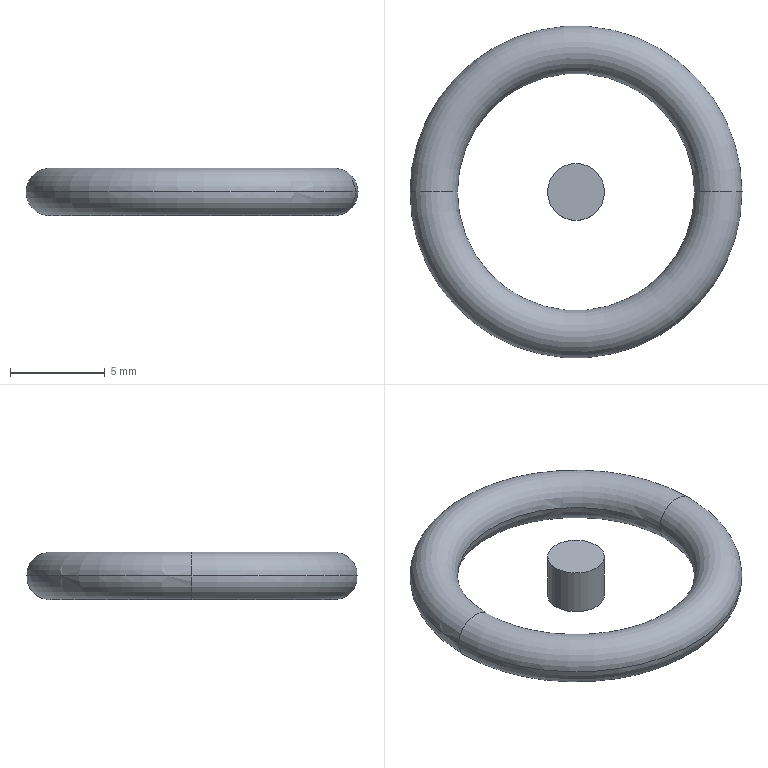Part | STEP file | O-ring 11 diameter after expansion | 2 solids | 8 faces | box 17.5 x 17.5 x 2.5 mm | volume 248.99 mm3 | torus 4 | cylinder 2 | plane 2 | commonest cylinder face diameters 3 x2
STEP:
#1=CARTESIAN_POINT('',(0.,0.,0.));
#2=DIRECTION('',(0.,0.,1.));
#3=DIRECTION('',(1.,0.,0.));
#4=AXIS2_PLACEMENT_3D('',#1,#2,#3);
#5=CARTESIAN_POINT('',(-8.75,0.,0.));
#6=VERTEX_POINT('',#5);
#7=CARTESIAN_POINT('',(-6.25,0.,0.));
#8=VERTEX_POINT('',#7);
#9=CARTESIAN_POINT('',(-7.5,0.,0.));
#10=DIRECTION('',(0.,1.,0.));
#11=DIRECTION('',(-1.,0.,0.));
#12=AXIS2_PLACEMENT_3D('',#9,#10,#11);
#13=CIRCLE('',#12,1.25);
#14=CARTESIAN_POINT('',(0.,0.,0.));
#15=DIRECTION('',(0.,0.,1.));
#16=DIRECTION('',(1.,0.,0.));
#17=AXIS2_PLACEMENT_3D('',#14,#15,#16);
#18=TOROIDAL_SURFACE('',#17,7.5,1.25);
#19=CARTESIAN_POINT('',(3.142,0.));
#20=DIRECTION('',(0.,1.));
#21=VECTOR('',#20,1.);
#22=LINE('',#19,#21);
#23=(GEOMETRIC_REPRESENTATION_CONTEXT(2)PARAMETRIC_REPRESENTATION_CONTEXT()REPRESENTATION_CONTEXT('',''));
#24=DEFINITIONAL_REPRESENTATION('',(#22),#23);
#25=PCURVE('',#18,#24);
#26=CARTESIAN_POINT('',(0.,0.,0.));
#27=DIRECTION('',(0.,0.,1.));
#28=DIRECTION('',(1.,0.,0.));
#29=AXIS2_PLACEMENT_3D('',#26,#27,#28);
#30=TOROIDAL_SURFACE('',#29,7.5,1.25);
#31=CARTESIAN_POINT('',(3.142,0.));
#32=DIRECTION('',(0.,1.));
#33=VECTOR('',#32,1.);
#34=LINE('',#31,#33);
#35=(GEOMETRIC_REPRESENTATION_CONTEXT(2)PARAMETRIC_REPRESENTATION_CONTEXT()REPRESENTATION_CONTEXT('',''));
#36=DEFINITIONAL_REPRESENTATION('',(#34),#35);
#37=PCURVE('',#30,#36);
#38=SURFACE_CURVE('',#13,(#25,#37),.PCURVE_S1.);
#39=EDGE_CURVE('',#6,#8,#38,.T.);
#40=ORIENTED_EDGE('',*,*,#39,.F.);
#41=CARTESIAN_POINT('',(8.75,0.,0.));
#42=VERTEX_POINT('',#41);
#43=CARTESIAN_POINT('',(0.,0.,0.));
#44=DIRECTION('',(0.,0.,1.));
#45=DIRECTION('',(1.,0.,0.));
#46=AXIS2_PLACEMENT_3D('',#43,#44,#45);
#47=CIRCLE('',#46,8.75);
#48=CARTESIAN_POINT('',(0.,0.));
#49=DIRECTION('',(1.,0.));
#50=VECTOR('',#49,1.);
#51=LINE('',#48,#50);
#52=(GEOMETRIC_REPRESENTATION_CONTEXT(2)PARAMETRIC_REPRESENTATION_CONTEXT()REPRESENTATION_CONTEXT('',''));
#53=DEFINITIONAL_REPRESENTATION('',(#51),#52);
#54=PCURVE('',#18,#53);
#55=CARTESIAN_POINT('',(0.,0.,0.));
#56=DIRECTION('',(0.,0.,1.));
#57=DIRECTION('',(1.,0.,0.));
#58=AXIS2_PLACEMENT_3D('',#55,#56,#57);
#59=TOROIDAL_SURFACE('',#58,7.5,1.25);
#60=CARTESIAN_POINT('',(0.,6.283));
#61=DIRECTION('',(1.,0.));
#62=VECTOR('',#61,1.);
#63=LINE('',#60,#62);
#64=(GEOMETRIC_REPRESENTATION_CONTEXT(2)PARAMETRIC_REPRESENTATION_CONTEXT()REPRESENTATION_CONTEXT('',''));
#65=DEFINITIONAL_REPRESENTATION('',(#63),#64);
#66=PCURVE('',#59,#65);
#67=SURFACE_CURVE('',#47,(#54,#66),.PCURVE_S1.);
#68=EDGE_CURVE('',#6,#42,#67,.T.);
#69=ORIENTED_EDGE('',*,*,#68,.T.);
#70=CARTESIAN_POINT('',(6.25,0.,0.));
#71=VERTEX_POINT('',#70);
#72=CARTESIAN_POINT('',(7.5,0.,0.));
#73=DIRECTION('',(0.,-1.,0.));
#74=DIRECTION('',(0.,0.,-1.));
#75=AXIS2_PLACEMENT_3D('',#72,#73,#74);
#76=CIRCLE('',#75,1.25);
#77=CARTESIAN_POINT('',(6.283,-1.571));
#78=DIRECTION('',(0.,1.));
#79=VECTOR('',#78,1.);
#80=LINE('',#77,#79);
#81=(GEOMETRIC_REPRESENTATION_CONTEXT(2)PARAMETRIC_REPRESENTATION_CONTEXT()REPRESENTATION_CONTEXT('',''));
#82=DEFINITIONAL_REPRESENTATION('',(#80),#81);
#83=PCURVE('',#18,#82);
#84=CARTESIAN_POINT('',(0.,-1.571));
#85=DIRECTION('',(0.,1.));
#86=VECTOR('',#85,1.);
#87=LINE('',#84,#86);
#88=(GEOMETRIC_REPRESENTATION_CONTEXT(2)PARAMETRIC_REPRESENTATION_CONTEXT()REPRESENTATION_CONTEXT('',''));
#89=DEFINITIONAL_REPRESENTATION('',(#87),#88);
#90=PCURVE('',#30,#89);
#91=SURFACE_CURVE('',#76,(#83,#90),.PCURVE_S1.);
#92=EDGE_CURVE('',#42,#71,#91,.T.);
#93=ORIENTED_EDGE('',*,*,#92,.T.);
#94=CARTESIAN_POINT('',(0.,0.,0.));
#95=DIRECTION('',(0.,0.,1.));
#96=DIRECTION('',(1.,0.,0.));
#97=AXIS2_PLACEMENT_3D('',#94,#95,#96);
#98=CIRCLE('',#97,6.25);
#99=CARTESIAN_POINT('',(0.,3.142));
#100=DIRECTION('',(1.,0.));
#101=VECTOR('',#100,1.);
#102=LINE('',#99,#101);
#103=(GEOMETRIC_REPRESENTATION_CONTEXT(2)PARAMETRIC_REPRESENTATION_CONTEXT()REPRESENTATION_CONTEXT('',''));
#104=DEFINITIONAL_REPRESENTATION('',(#102),#103);
#105=PCURVE('',#18,#104);
#106=CARTESIAN_POINT('',(0.,3.142));
#107=DIRECTION('',(1.,0.));
#108=VECTOR('',#107,1.);
#109=LINE('',#106,#108);
#110=(GEOMETRIC_REPRESENTATION_CONTEXT(2)PARAMETRIC_REPRESENTATION_CONTEXT()REPRESENTATION_CONTEXT('',''));
#111=DEFINITIONAL_REPRESENTATION('',(#109),#110);
#112=PCURVE('',#59,#111);
#113=SURFACE_CURVE('',#98,(#105,#112),.PCURVE_S1.);
#114=EDGE_CURVE('',#8,#71,#113,.T.);
#115=ORIENTED_EDGE('',*,*,#114,.F.);
#116=EDGE_LOOP('',(#40,#69,#93,#115));
#117=FACE_BOUND('',#116,.T.);
#118=ADVANCED_FACE('',(#117),#18,.T.);
#119=ORIENTED_EDGE('',*,*,#92,.F.);
#120=CARTESIAN_POINT('',(0.,0.,0.));
#121=DIRECTION('',(0.,0.,1.));
#122=DIRECTION('',(1.,0.,0.));
#123=AXIS2_PLACEMENT_3D('',#120,#121,#122);
#124=CIRCLE('',#123,8.75);
#125=CARTESIAN_POINT('',(0.,0.));
#126=DIRECTION('',(1.,0.));
#127=VECTOR('',#126,1.);
#128=LINE('',#125,#127);
#129=(GEOMETRIC_REPRESENTATION_CONTEXT(2)PARAMETRIC_REPRESENTATION_CONTEXT()REPRESENTATION_CONTEXT('',''));
#130=DEFINITIONAL_REPRESENTATION('',(#128),#129);
#131=PCURVE('',#30,#130);
#132=CARTESIAN_POINT('',(0.,0.,0.));
#133=DIRECTION('',(0.,0.,1.));
#134=DIRECTION('',(1.,0.,0.));
#135=AXIS2_PLACEMENT_3D('',#132,#133,#134);
#136=TOROIDAL_SURFACE('',#135,7.5,1.25);
#137=CARTESIAN_POINT('',(0.,6.283));
#138=DIRECTION('',(1.,0.));
#139=VECTOR('',#138,1.);
#140=LINE('',#137,#139);
#141=(GEOMETRIC_REPRESENTATION_CONTEXT(2)PARAMETRIC_REPRESENTATION_CONTEXT()REPRESENTATION_CONTEXT('',''));
#142=DEFINITIONAL_REPRESENTATION('',(#140),#141);
#143=PCURVE('',#136,#142);
#144=SURFACE_CURVE('',#124,(#131,#143),.PCURVE_S1.);
#145=EDGE_CURVE('',#42,#6,#144,.T.);
#146=ORIENTED_EDGE('',*,*,#145,.T.);
#147=ORIENTED_EDGE('',*,*,#39,.T.);
#148=CARTESIAN_POINT('',(0.,0.,0.));
#149=DIRECTION('',(0.,0.,1.));
#150=DIRECTION('',(1.,0.,0.));
#151=AXIS2_PLACEMENT_3D('',#148,#149,#150);
#152=CIRCLE('',#151,6.25);
#153=CARTESIAN_POINT('',(0.,3.142));
#154=DIRECTION('',(1.,0.));
#155=VECTOR('',#154,1.);
#156=LINE('',#153,#155);
#157=(GEOMETRIC_REPRESENTATION_CONTEXT(2)PARAMETRIC_REPRESENTATION_CONTEXT()REPRESENTATION_CONTEXT('',''));
#158=DEFINITIONAL_REPRESENTATION('',(#156),#157);
#159=PCURVE('',#30,#158);
#160=CARTESIAN_POINT('',(0.,3.142));
#161=DIRECTION('',(1.,0.));
#162=VECTOR('',#161,1.);
#163=LINE('',#160,#162);
#164=(GEOMETRIC_REPRESENTATION_CONTEXT(2)PARAMETRIC_REPRESENTATION_CONTEXT()REPRESENTATION_CONTEXT('',''));
#165=DEFINITIONAL_REPRESENTATION('',(#163),#164);
#166=PCURVE('',#136,#165);
#167=SURFACE_CURVE('',#152,(#159,#166),.PCURVE_S1.);
#168=EDGE_CURVE('',#71,#8,#167,.T.);
#169=ORIENTED_EDGE('',*,*,#168,.F.);
#170=EDGE_LOOP('',(#119,#146,#147,#169));
#171=FACE_BOUND('',#170,.T.);
#172=ADVANCED_FACE('',(#171),#30,.T.);
#173=ORIENTED_EDGE('',*,*,#145,.F.);
#174=CARTESIAN_POINT('',(7.5,0.,0.));
#175=DIRECTION('',(0.,-1.,0.));
#176=DIRECTION('',(0.,0.,-1.));
#177=AXIS2_PLACEMENT_3D('',#174,#175,#176);
#178=CIRCLE('',#177,1.25);
#179=CARTESIAN_POINT('',(0.,-1.571));
#180=DIRECTION('',(0.,1.));
#181=VECTOR('',#180,1.);
#182=LINE('',#179,#181);
#183=(GEOMETRIC_REPRESENTATION_CONTEXT(2)PARAMETRIC_REPRESENTATION_CONTEXT()REPRESENTATION_CONTEXT('',''));
#184=DEFINITIONAL_REPRESENTATION('',(#182),#183);
#185=PCURVE('',#136,#184);
#186=CARTESIAN_POINT('',(6.283,-1.571));
#187=DIRECTION('',(0.,1.));
#188=VECTOR('',#187,1.);
#189=LINE('',#186,#188);
#190=(GEOMETRIC_REPRESENTATION_CONTEXT(2)PARAMETRIC_REPRESENTATION_CONTEXT()REPRESENTATION_CONTEXT('',''));
#191=DEFINITIONAL_REPRESENTATION('',(#189),#190);
#192=PCURVE('',#59,#191);
#193=SURFACE_CURVE('',#178,(#185,#192),.PCURVE_S1.);
#194=EDGE_CURVE('',#71,#42,#193,.T.);
#195=ORIENTED_EDGE('',*,*,#194,.F.);
#196=ORIENTED_EDGE('',*,*,#168,.T.);
#197=CARTESIAN_POINT('',(-7.5,0.,0.));
#198=DIRECTION('',(0.,1.,0.));
#199=DIRECTION('',(-1.,0.,0.));
#200=AXIS2_PLACEMENT_3D('',#197,#198,#199);
#201=CIRCLE('',#200,1.25);
#202=CARTESIAN_POINT('',(3.142,0.));
#203=DIRECTION('',(0.,1.));
#204=VECTOR('',#203,1.);
#205=LINE('',#202,#204);
#206=(GEOMETRIC_REPRESENTATION_CONTEXT(2)PARAMETRIC_REPRESENTATION_CONTEXT()REPRESENTATION_CONTEXT('',''));
#207=DEFINITIONAL_REPRESENTATION('',(#205),#206);
#208=PCURVE('',#136,#207);
#209=CARTESIAN_POINT('',(3.142,0.));
#210=DIRECTION('',(0.,1.));
#211=VECTOR('',#210,1.);
#212=LINE('',#209,#211);
#213=(GEOMETRIC_REPRESENTATION_CONTEXT(2)PARAMETRIC_REPRESENTATION_CONTEXT()REPRESENTATION_CONTEXT('',''));
#214=DEFINITIONAL_REPRESENTATION('',(#212),#213);
#215=PCURVE('',#59,#214);
#216=SURFACE_CURVE('',#201,(#208,#215),.PCURVE_S1.);
#217=EDGE_CURVE('',#8,#6,#216,.T.);
#218=ORIENTED_EDGE('',*,*,#217,.T.);
#219=EDGE_LOOP('',(#173,#195,#196,#218));
#220=FACE_BOUND('',#219,.T.);
#221=ADVANCED_FACE('',(#220),#136,.T.);
#222=ORIENTED_EDGE('',*,*,#68,.F.);
#223=ORIENTED_EDGE('',*,*,#217,.F.);
#224=ORIENTED_EDGE('',*,*,#114,.T.);
#225=ORIENTED_EDGE('',*,*,#194,.T.);
#226=EDGE_LOOP('',(#222,#223,#224,#225));
#227=FACE_BOUND('',#226,.T.);
#228=ADVANCED_FACE('',(#227),#59,.T.);
#229=CLOSED_SHELL('',(#118,#172,#221,#228));
#230=MANIFOLD_SOLID_BREP('',#229);
#231=CARTESIAN_POINT('',(1.5,0.,-1.25));
#232=VERTEX_POINT('',#231);
#233=CARTESIAN_POINT('',(-1.5,0.,-1.25));
#234=VERTEX_POINT('',#233);
#235=CARTESIAN_POINT('',(0.,0.,-1.25));
#236=DIRECTION('',(0.,0.,1.));
#237=DIRECTION('',(1.,0.,0.));
#238=AXIS2_PLACEMENT_3D('',#235,#236,#237);
#239=CIRCLE('',#238,1.5);
#240=CARTESIAN_POINT('',(0.,0.,-1.25));
#241=DIRECTION('',(0.,0.,1.));
#242=DIRECTION('',(1.,0.,0.));
#243=AXIS2_PLACEMENT_3D('',#240,#241,#242);
#244=CYLINDRICAL_SURFACE('',#243,1.5);
#245=CARTESIAN_POINT('',(0.,0.));
#246=DIRECTION('',(1.,0.));
#247=VECTOR('',#246,1.);
#248=LINE('',#245,#247);
#249=(GEOMETRIC_REPRESENTATION_CONTEXT(2)PARAMETRIC_REPRESENTATION_CONTEXT()REPRESENTATION_CONTEXT('',''));
#250=DEFINITIONAL_REPRESENTATION('',(#248),#249);
#251=PCURVE('',#244,#250);
#252=CARTESIAN_POINT('',(0.,0.,-1.25));
#253=DIRECTION('',(0.,0.,1.));
#254=DIRECTION('',(1.,0.,0.));
#255=AXIS2_PLACEMENT_3D('',#252,#253,#254);
#256=PLANE('',#255);
#257=CARTESIAN_POINT('',(0.,0.));
#258=DIRECTION('',(1.,0.));
#259=AXIS2_PLACEMENT_2D('',#257,#258);
#260=CIRCLE('',#259,1.5);
#261=(GEOMETRIC_REPRESENTATION_CONTEXT(2)PARAMETRIC_REPRESENTATION_CONTEXT()REPRESENTATION_CONTEXT('',''));
#262=DEFINITIONAL_REPRESENTATION('',(#260),#261);
#263=PCURVE('',#256,#262);
#264=SURFACE_CURVE('',#239,(#251,#263),.PCURVE_S1.);
#265=EDGE_CURVE('',#232,#234,#264,.T.);
#266=ORIENTED_EDGE('',*,*,#265,.T.);
#267=CARTESIAN_POINT('',(-1.5,0.,1.25));
#268=VERTEX_POINT('',#267);
#269=CARTESIAN_POINT('',(-1.5,0.,-1.25));
#270=DIRECTION('',(0.,0.,1.));
#271=VECTOR('',#270,1.);
#272=LINE('',#269,#271);
#273=CARTESIAN_POINT('',(3.142,0.));
#274=DIRECTION('',(0.,1.));
#275=VECTOR('',#274,1.);
#276=LINE('',#273,#275);
#277=(GEOMETRIC_REPRESENTATION_CONTEXT(2)PARAMETRIC_REPRESENTATION_CONTEXT()REPRESENTATION_CONTEXT('',''));
#278=DEFINITIONAL_REPRESENTATION('',(#276),#277);
#279=PCURVE('',#244,#278);
#280=CARTESIAN_POINT('',(0.,0.,-1.25));
#281=DIRECTION('',(0.,0.,1.));
#282=DIRECTION('',(1.,0.,0.));
#283=AXIS2_PLACEMENT_3D('',#280,#281,#282);
#284=CYLINDRICAL_SURFACE('',#283,1.5);
#285=CARTESIAN_POINT('',(3.142,0.));
#286=DIRECTION('',(0.,1.));
#287=VECTOR('',#286,1.);
#288=LINE('',#285,#287);
#289=(GEOMETRIC_REPRESENTATION_CONTEXT(2)PARAMETRIC_REPRESENTATION_CONTEXT()REPRESENTATION_CONTEXT('',''));
#290=DEFINITIONAL_REPRESENTATION('',(#288),#289);
#291=PCURVE('',#284,#290);
#292=SURFACE_CURVE('',#272,(#279,#291),.PCURVE_S1.);
#293=EDGE_CURVE('',#234,#268,#292,.T.);
#294=ORIENTED_EDGE('',*,*,#293,.T.);
#295=CARTESIAN_POINT('',(1.5,0.,1.25));
#296=VERTEX_POINT('',#295);
#297=CARTESIAN_POINT('',(0.,0.,1.25));
#298=DIRECTION('',(0.,0.,1.));
#299=DIRECTION('',(1.,0.,0.));
#300=AXIS2_PLACEMENT_3D('',#297,#298,#299);
#301=CIRCLE('',#300,1.5);
#302=CARTESIAN_POINT('',(0.,2.5));
#303=DIRECTION('',(1.,0.));
#304=VECTOR('',#303,1.);
#305=LINE('',#302,#304);
#306=(GEOMETRIC_REPRESENTATION_CONTEXT(2)PARAMETRIC_REPRESENTATION_CONTEXT()REPRESENTATION_CONTEXT('',''));
#307=DEFINITIONAL_REPRESENTATION('',(#305),#306);
#308=PCURVE('',#244,#307);
#309=CARTESIAN_POINT('',(0.,0.,1.25));
#310=DIRECTION('',(0.,0.,1.));
#311=DIRECTION('',(1.,0.,0.));
#312=AXIS2_PLACEMENT_3D('',#309,#310,#311);
#313=PLANE('',#312);
#314=CARTESIAN_POINT('',(0.,0.));
#315=DIRECTION('',(1.,0.));
#316=AXIS2_PLACEMENT_2D('',#314,#315);
#317=CIRCLE('',#316,1.5);
#318=(GEOMETRIC_REPRESENTATION_CONTEXT(2)PARAMETRIC_REPRESENTATION_CONTEXT()REPRESENTATION_CONTEXT('',''));
#319=DEFINITIONAL_REPRESENTATION('',(#317),#318);
#320=PCURVE('',#313,#319);
#321=SURFACE_CURVE('',#301,(#308,#320),.PCURVE_S1.);
#322=EDGE_CURVE('',#296,#268,#321,.T.);
#323=ORIENTED_EDGE('',*,*,#322,.F.);
#324=CARTESIAN_POINT('',(1.5,0.,-1.25));
#325=DIRECTION('',(0.,0.,1.));
#326=VECTOR('',#325,1.);
#327=LINE('',#324,#326);
#328=CARTESIAN_POINT('',(0.,0.));
#329=DIRECTION('',(0.,1.));
#330=VECTOR('',#329,1.);
#331=LINE('',#328,#330);
#332=(GEOMETRIC_REPRESENTATION_CONTEXT(2)PARAMETRIC_REPRESENTATION_CONTEXT()REPRESENTATION_CONTEXT('',''));
#333=DEFINITIONAL_REPRESENTATION('',(#331),#332);
#334=PCURVE('',#244,#333);
#335=CARTESIAN_POINT('',(6.283,0.));
#336=DIRECTION('',(0.,1.));
#337=VECTOR('',#336,1.);
#338=LINE('',#335,#337);
#339=(GEOMETRIC_REPRESENTATION_CONTEXT(2)PARAMETRIC_REPRESENTATION_CONTEXT()REPRESENTATION_CONTEXT('',''));
#340=DEFINITIONAL_REPRESENTATION('',(#338),#339);
#341=PCURVE('',#284,#340);
#342=SURFACE_CURVE('',#327,(#334,#341),.PCURVE_S1.);
#343=EDGE_CURVE('',#232,#296,#342,.T.);
#344=ORIENTED_EDGE('',*,*,#343,.F.);
#345=EDGE_LOOP('',(#266,#294,#323,#344));
#346=FACE_BOUND('',#345,.T.);
#347=ADVANCED_FACE('',(#346),#244,.T.);
#348=ORIENTED_EDGE('',*,*,#293,.F.);
#349=CARTESIAN_POINT('',(0.,0.,-1.25));
#350=DIRECTION('',(0.,0.,1.));
#351=DIRECTION('',(1.,0.,0.));
#352=AXIS2_PLACEMENT_3D('',#349,#350,#351);
#353=CIRCLE('',#352,1.5);
#354=CARTESIAN_POINT('',(0.,0.));
#355=DIRECTION('',(1.,0.));
#356=VECTOR('',#355,1.);
#357=LINE('',#354,#356);
#358=(GEOMETRIC_REPRESENTATION_CONTEXT(2)PARAMETRIC_REPRESENTATION_CONTEXT()REPRESENTATION_CONTEXT('',''));
#359=DEFINITIONAL_REPRESENTATION('',(#357),#358);
#360=PCURVE('',#284,#359);
#361=CARTESIAN_POINT('',(0.,0.));
#362=DIRECTION('',(1.,0.));
#363=AXIS2_PLACEMENT_2D('',#361,#362);
#364=CIRCLE('',#363,1.5);
#365=(GEOMETRIC_REPRESENTATION_CONTEXT(2)PARAMETRIC_REPRESENTATION_CONTEXT()REPRESENTATION_CONTEXT('',''));
#366=DEFINITIONAL_REPRESENTATION('',(#364),#365);
#367=PCURVE('',#256,#366);
#368=SURFACE_CURVE('',#353,(#360,#367),.PCURVE_S1.);
#369=EDGE_CURVE('',#234,#232,#368,.T.);
#370=ORIENTED_EDGE('',*,*,#369,.T.);
#371=ORIENTED_EDGE('',*,*,#343,.T.);
#372=CARTESIAN_POINT('',(0.,0.,1.25));
#373=DIRECTION('',(0.,0.,1.));
#374=DIRECTION('',(1.,0.,0.));
#375=AXIS2_PLACEMENT_3D('',#372,#373,#374);
#376=CIRCLE('',#375,1.5);
#377=CARTESIAN_POINT('',(0.,2.5));
#378=DIRECTION('',(1.,0.));
#379=VECTOR('',#378,1.);
#380=LINE('',#377,#379);
#381=(GEOMETRIC_REPRESENTATION_CONTEXT(2)PARAMETRIC_REPRESENTATION_CONTEXT()REPRESENTATION_CONTEXT('',''));
#382=DEFINITIONAL_REPRESENTATION('',(#380),#381);
#383=PCURVE('',#284,#382);
#384=CARTESIAN_POINT('',(0.,0.));
#385=DIRECTION('',(1.,0.));
#386=AXIS2_PLACEMENT_2D('',#384,#385);
#387=CIRCLE('',#386,1.5);
#388=(GEOMETRIC_REPRESENTATION_CONTEXT(2)PARAMETRIC_REPRESENTATION_CONTEXT()REPRESENTATION_CONTEXT('',''));
#389=DEFINITIONAL_REPRESENTATION('',(#387),#388);
#390=PCURVE('',#313,#389);
#391=SURFACE_CURVE('',#376,(#383,#390),.PCURVE_S1.);
#392=EDGE_CURVE('',#268,#296,#391,.T.);
#393=ORIENTED_EDGE('',*,*,#392,.F.);
#394=EDGE_LOOP('',(#348,#370,#371,#393));
#395=FACE_BOUND('',#394,.T.);
#396=ADVANCED_FACE('',(#395),#284,.T.);
#397=ORIENTED_EDGE('',*,*,#265,.F.);
#398=ORIENTED_EDGE('',*,*,#369,.F.);
#399=EDGE_LOOP('',(#397,#398));
#400=FACE_BOUND('',#399,.T.);
#401=ADVANCED_FACE('',(#400),#256,.F.);
#402=ORIENTED_EDGE('',*,*,#322,.T.);
#403=ORIENTED_EDGE('',*,*,#392,.T.);
#404=EDGE_LOOP('',(#402,#403));
#405=FACE_BOUND('',#404,.T.);
#406=ADVANCED_FACE('',(#405),#313,.T.);
#407=CLOSED_SHELL('',(#347,#396,#401,#406));
#408=MANIFOLD_SOLID_BREP('',#407);
#409=(LENGTH_UNIT()NAMED_UNIT(*)SI_UNIT(.MILLI.,.METRE.));
#410=UNCERTAINTY_MEASURE_WITH_UNIT(LENGTH_MEASURE(0.0000001),#409,'','');
#411=(NAMED_UNIT(*)PLANE_ANGLE_UNIT()SI_UNIT($,.RADIAN.));
#412=(NAMED_UNIT(*)SI_UNIT($,.STERADIAN.)SOLID_ANGLE_UNIT());
#413=(GEOMETRIC_REPRESENTATION_CONTEXT(3)GLOBAL_UNCERTAINTY_ASSIGNED_CONTEXT((#410))GLOBAL_UNIT_ASSIGNED_CONTEXT((#409,#411,#412))REPRESENTATION_CONTEXT('',''));
#414=SHAPE_REPRESENTATION('',(#4,#230,#408),#413);